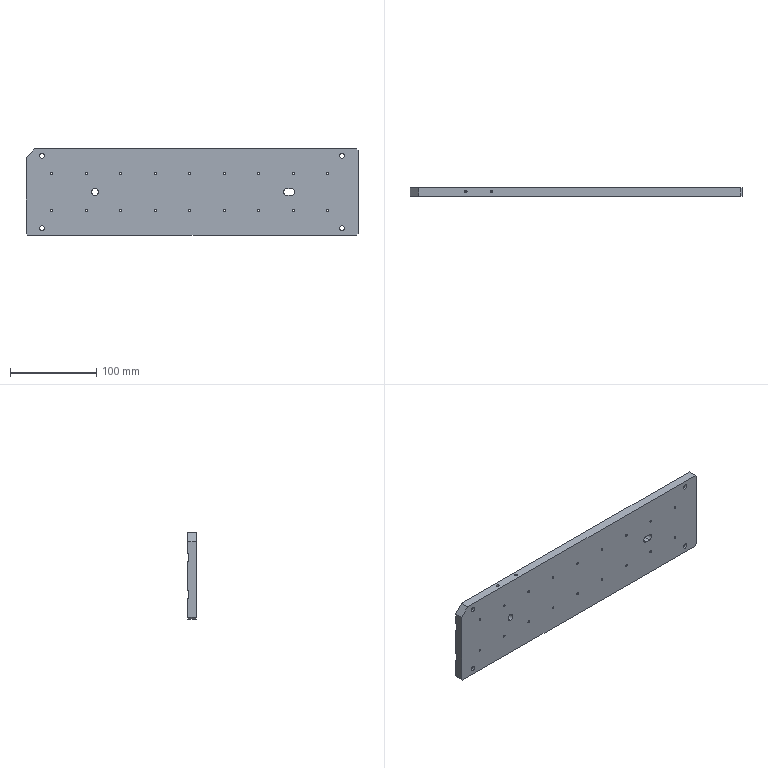Part | SolidWorks | features ICE 5, Chamfer 2, HoleWzd 2, 3DProfileFeature 1, Extrusion 1, LPattern 1 | 1 solid | 88 faces | box 385 x 10 x 100 mm | volume 371645 mm3 | cylinder 60 | plane 24 | cone 4 | commonest cylinder face diameters 2.5 x36 5.5 x8 12 x8 3.3 x4 8 x4